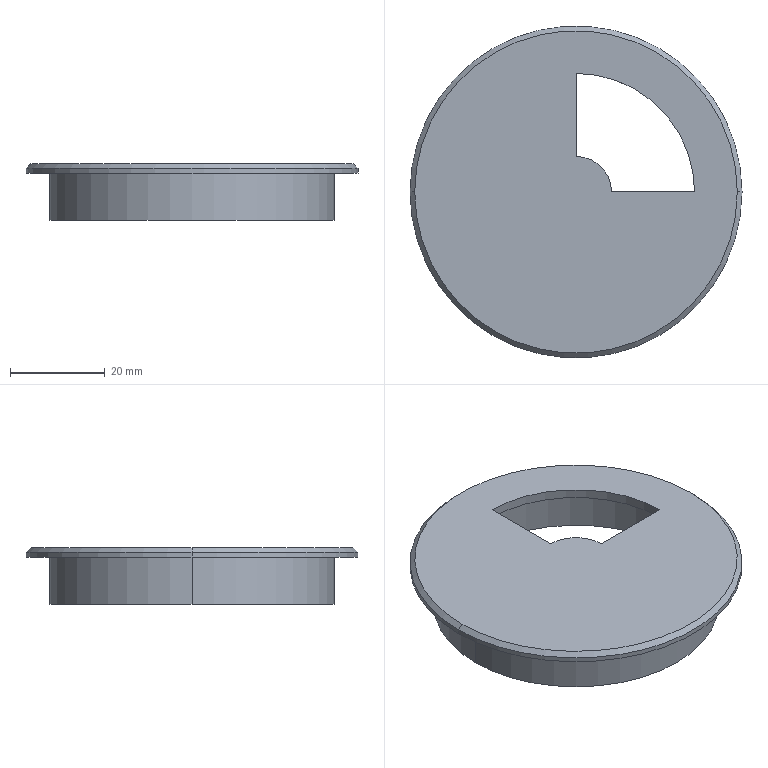Part | STEP file | 1 solid | 16 faces | box 70 x 70 x 12 mm | volume 8548 mm3 | cylinder 8 | plane 6 | cone 2 | commonest cylinder face diameters 58 x2 60 x2 70 x2 15 x1 50 x1
STEP:
#1=CARTESIAN_POINT('',(0.,0.,0.));
#2=DIRECTION('',(0.,0.,1.));
#3=DIRECTION('',(1.,0.,0.));
#4=AXIS2_PLACEMENT_3D('',#1,#2,#3);
#5=CARTESIAN_POINT('',(34.,0.,12.));
#6=VERTEX_POINT('',#5);
#7=CARTESIAN_POINT('',(-34.,0.,12.));
#8=VERTEX_POINT('',#7);
#9=CARTESIAN_POINT('',(0.,0.,12.));
#10=DIRECTION('',(0.,0.,1.));
#11=DIRECTION('',(1.,0.,0.));
#12=AXIS2_PLACEMENT_3D('',#9,#10,#11);
#13=CIRCLE('',#12,34.);
#14=CARTESIAN_POINT('',(0.,0.,12.));
#15=DIRECTION('',(0.,0.,-1.));
#16=DIRECTION('',(-1.,0.,0.));
#17=AXIS2_PLACEMENT_3D('',#14,#15,#16);
#18=CONICAL_SURFACE('',#17,34.,0.7854);
#19=CARTESIAN_POINT('',(3.142,0.));
#20=DIRECTION('',(-1.,0.));
#21=VECTOR('',#20,1.);
#22=LINE('',#19,#21);
#23=(GEOMETRIC_REPRESENTATION_CONTEXT(2)PARAMETRIC_REPRESENTATION_CONTEXT()REPRESENTATION_CONTEXT('',''));
#24=DEFINITIONAL_REPRESENTATION('',(#22),#23);
#25=PCURVE('',#18,#24);
#26=CARTESIAN_POINT('',(0.,0.,12.));
#27=DIRECTION('',(0.,0.,1.));
#28=DIRECTION('',(1.,0.,0.));
#29=AXIS2_PLACEMENT_3D('',#26,#27,#28);
#30=PLANE('',#29);
#31=CARTESIAN_POINT('',(0.,0.));
#32=DIRECTION('',(1.,0.));
#33=AXIS2_PLACEMENT_2D('',#31,#32);
#34=CIRCLE('',#33,34.);
#35=(GEOMETRIC_REPRESENTATION_CONTEXT(2)PARAMETRIC_REPRESENTATION_CONTEXT()REPRESENTATION_CONTEXT('',''));
#36=DEFINITIONAL_REPRESENTATION('',(#34),#35);
#37=PCURVE('',#30,#36);
#38=SURFACE_CURVE('',#13,(#25,#37),.PCURVE_S1.);
#39=EDGE_CURVE('',#6,#8,#38,.T.);
#40=ORIENTED_EDGE('',*,*,#39,.F.);
#41=CARTESIAN_POINT('',(35.,0.,11.));
#42=VERTEX_POINT('',#41);
#43=CARTESIAN_POINT('',(34.,0.,12.));
#44=DIRECTION('',(0.7071,0.,-0.7071));
#45=VECTOR('',#44,1.);
#46=LINE('',#43,#45);
#47=CARTESIAN_POINT('',(3.142,0.));
#48=DIRECTION('',(0.,1.));
#49=VECTOR('',#48,1.);
#50=LINE('',#47,#49);
#51=(GEOMETRIC_REPRESENTATION_CONTEXT(2)PARAMETRIC_REPRESENTATION_CONTEXT()REPRESENTATION_CONTEXT('',''));
#52=DEFINITIONAL_REPRESENTATION('',(#50),#51);
#53=PCURVE('',#18,#52);
#54=CARTESIAN_POINT('',(0.,0.,12.));
#55=DIRECTION('',(0.,0.,-1.));
#56=DIRECTION('',(-1.,0.,0.));
#57=AXIS2_PLACEMENT_3D('',#54,#55,#56);
#58=CONICAL_SURFACE('',#57,34.,0.7854);
#59=CARTESIAN_POINT('',(3.142,0.));
#60=DIRECTION('',(0.,1.));
#61=VECTOR('',#60,1.);
#62=LINE('',#59,#61);
#63=(GEOMETRIC_REPRESENTATION_CONTEXT(2)PARAMETRIC_REPRESENTATION_CONTEXT()REPRESENTATION_CONTEXT('',''));
#64=DEFINITIONAL_REPRESENTATION('',(#62),#63);
#65=PCURVE('',#58,#64);
#66=SURFACE_CURVE('',#46,(#53,#65),.PCURVE_S1.);
#67=EDGE_CURVE('',#6,#42,#66,.T.);
#68=ORIENTED_EDGE('',*,*,#67,.T.);
#69=CARTESIAN_POINT('',(-35.,0.,11.));
#70=VERTEX_POINT('',#69);
#71=CARTESIAN_POINT('',(0.,0.,11.));
#72=DIRECTION('',(0.,0.,-1.));
#73=DIRECTION('',(1.,0.,0.));
#74=AXIS2_PLACEMENT_3D('',#71,#72,#73);
#75=CIRCLE('',#74,35.);
#76=CARTESIAN_POINT('',(-3.142,1.));
#77=DIRECTION('',(1.,0.));
#78=VECTOR('',#77,1.);
#79=LINE('',#76,#78);
#80=(GEOMETRIC_REPRESENTATION_CONTEXT(2)PARAMETRIC_REPRESENTATION_CONTEXT()REPRESENTATION_CONTEXT('',''));
#81=DEFINITIONAL_REPRESENTATION('',(#79),#80);
#82=PCURVE('',#18,#81);
#83=CARTESIAN_POINT('',(0.,0.,12.));
#84=DIRECTION('',(0.,0.,-1.));
#85=DIRECTION('',(-1.,0.,0.));
#86=AXIS2_PLACEMENT_3D('',#83,#84,#85);
#87=CYLINDRICAL_SURFACE('',#86,35.);
#88=CARTESIAN_POINT('',(-3.142,1.));
#89=DIRECTION('',(1.,0.));
#90=VECTOR('',#89,1.);
#91=LINE('',#88,#90);
#92=(GEOMETRIC_REPRESENTATION_CONTEXT(2)PARAMETRIC_REPRESENTATION_CONTEXT()REPRESENTATION_CONTEXT('',''));
#93=DEFINITIONAL_REPRESENTATION('',(#91),#92);
#94=PCURVE('',#87,#93);
#95=SURFACE_CURVE('',#75,(#82,#94),.PCURVE_S1.);
#96=EDGE_CURVE('',#70,#42,#95,.T.);
#97=ORIENTED_EDGE('',*,*,#96,.F.);
#98=CARTESIAN_POINT('',(-34.,0.,12.));
#99=DIRECTION('',(-0.7071,0.,-0.7071));
#100=VECTOR('',#99,1.);
#101=LINE('',#98,#100);
#102=CARTESIAN_POINT('',(0.,0.));
#103=DIRECTION('',(0.,1.));
#104=VECTOR('',#103,1.);
#105=LINE('',#102,#104);
#106=(GEOMETRIC_REPRESENTATION_CONTEXT(2)PARAMETRIC_REPRESENTATION_CONTEXT()REPRESENTATION_CONTEXT('',''));
#107=DEFINITIONAL_REPRESENTATION('',(#105),#106);
#108=PCURVE('',#18,#107);
#109=CARTESIAN_POINT('',(6.283,0.));
#110=DIRECTION('',(0.,1.));
#111=VECTOR('',#110,1.);
#112=LINE('',#109,#111);
#113=(GEOMETRIC_REPRESENTATION_CONTEXT(2)PARAMETRIC_REPRESENTATION_CONTEXT()REPRESENTATION_CONTEXT('',''));
#114=DEFINITIONAL_REPRESENTATION('',(#112),#113);
#115=PCURVE('',#58,#114);
#116=SURFACE_CURVE('',#101,(#108,#115),.PCURVE_S1.);
#117=EDGE_CURVE('',#8,#70,#116,.T.);
#118=ORIENTED_EDGE('',*,*,#117,.F.);
#119=EDGE_LOOP('',(#40,#68,#97,#118));
#120=FACE_BOUND('',#119,.T.);
#121=ADVANCED_FACE('',(#120),#18,.T.);
#122=ORIENTED_EDGE('',*,*,#96,.T.);
#123=CARTESIAN_POINT('',(35.,0.,10.));
#124=VERTEX_POINT('',#123);
#125=CARTESIAN_POINT('',(35.,0.,12.));
#126=DIRECTION('',(0.,0.,-1.));
#127=VECTOR('',#126,1.);
#128=LINE('',#125,#127);
#129=CARTESIAN_POINT('',(3.142,0.));
#130=DIRECTION('',(0.,1.));
#131=VECTOR('',#130,1.);
#132=LINE('',#129,#131);
#133=(GEOMETRIC_REPRESENTATION_CONTEXT(2)PARAMETRIC_REPRESENTATION_CONTEXT()REPRESENTATION_CONTEXT('',''));
#134=DEFINITIONAL_REPRESENTATION('',(#132),#133);
#135=PCURVE('',#87,#134);
#136=CARTESIAN_POINT('',(0.,0.,12.));
#137=DIRECTION('',(0.,0.,-1.));
#138=DIRECTION('',(-1.,0.,0.));
#139=AXIS2_PLACEMENT_3D('',#136,#137,#138);
#140=CYLINDRICAL_SURFACE('',#139,35.);
#141=CARTESIAN_POINT('',(3.142,0.));
#142=DIRECTION('',(0.,1.));
#143=VECTOR('',#142,1.);
#144=LINE('',#141,#143);
#145=(GEOMETRIC_REPRESENTATION_CONTEXT(2)PARAMETRIC_REPRESENTATION_CONTEXT()REPRESENTATION_CONTEXT('',''));
#146=DEFINITIONAL_REPRESENTATION('',(#144),#145);
#147=PCURVE('',#140,#146);
#148=SURFACE_CURVE('',#128,(#135,#147),.PCURVE_S1.);
#149=EDGE_CURVE('',#42,#124,#148,.T.);
#150=ORIENTED_EDGE('',*,*,#149,.T.);
#151=CARTESIAN_POINT('',(-35.,0.,10.));
#152=VERTEX_POINT('',#151);
#153=CARTESIAN_POINT('',(0.,0.,10.));
#154=DIRECTION('',(0.,0.,1.));
#155=DIRECTION('',(1.,0.,0.));
#156=AXIS2_PLACEMENT_3D('',#153,#154,#155);
#157=CIRCLE('',#156,35.);
#158=CARTESIAN_POINT('',(3.142,2.));
#159=DIRECTION('',(-1.,0.));
#160=VECTOR('',#159,1.);
#161=LINE('',#158,#160);
#162=(GEOMETRIC_REPRESENTATION_CONTEXT(2)PARAMETRIC_REPRESENTATION_CONTEXT()REPRESENTATION_CONTEXT('',''));
#163=DEFINITIONAL_REPRESENTATION('',(#161),#162);
#164=PCURVE('',#87,#163);
#165=CARTESIAN_POINT('',(0.,0.,10.));
#166=DIRECTION('',(0.,0.,1.));
#167=DIRECTION('',(1.,0.,0.));
#168=AXIS2_PLACEMENT_3D('',#165,#166,#167);
#169=PLANE('',#168);
#170=CARTESIAN_POINT('',(0.,0.));
#171=DIRECTION('',(1.,0.));
#172=AXIS2_PLACEMENT_2D('',#170,#171);
#173=CIRCLE('',#172,35.);
#174=(GEOMETRIC_REPRESENTATION_CONTEXT(2)PARAMETRIC_REPRESENTATION_CONTEXT()REPRESENTATION_CONTEXT('',''));
#175=DEFINITIONAL_REPRESENTATION('',(#173),#174);
#176=PCURVE('',#169,#175);
#177=SURFACE_CURVE('',#157,(#164,#176),.PCURVE_S1.);
#178=EDGE_CURVE('',#124,#152,#177,.T.);
#179=ORIENTED_EDGE('',*,*,#178,.T.);
#180=CARTESIAN_POINT('',(-35.,0.,12.));
#181=DIRECTION('',(0.,0.,-1.));
#182=VECTOR('',#181,1.);
#183=LINE('',#180,#182);
#184=CARTESIAN_POINT('',(0.,0.));
#185=DIRECTION('',(0.,1.));
#186=VECTOR('',#185,1.);
#187=LINE('',#184,#186);
#188=(GEOMETRIC_REPRESENTATION_CONTEXT(2)PARAMETRIC_REPRESENTATION_CONTEXT()REPRESENTATION_CONTEXT('',''));
#189=DEFINITIONAL_REPRESENTATION('',(#187),#188);
#190=PCURVE('',#87,#189);
#191=CARTESIAN_POINT('',(6.283,0.));
#192=DIRECTION('',(0.,1.));
#193=VECTOR('',#192,1.);
#194=LINE('',#191,#193);
#195=(GEOMETRIC_REPRESENTATION_CONTEXT(2)PARAMETRIC_REPRESENTATION_CONTEXT()REPRESENTATION_CONTEXT('',''));
#196=DEFINITIONAL_REPRESENTATION('',(#194),#195);
#197=PCURVE('',#140,#196);
#198=SURFACE_CURVE('',#183,(#190,#197),.PCURVE_S1.);
#199=EDGE_CURVE('',#70,#152,#198,.T.);
#200=ORIENTED_EDGE('',*,*,#199,.F.);
#201=EDGE_LOOP('',(#122,#150,#179,#200));
#202=FACE_BOUND('',#201,.T.);
#203=ADVANCED_FACE('',(#202),#87,.T.);
#204=CARTESIAN_POINT('',(-29.,0.,10.));
#205=VERTEX_POINT('',#204);
#206=CARTESIAN_POINT('',(-29.,0.,0.));
#207=VERTEX_POINT('',#206);
#208=CARTESIAN_POINT('',(-29.,0.,10.));
#209=DIRECTION('',(0.,0.,-1.));
#210=VECTOR('',#209,1.);
#211=LINE('',#208,#210);
#212=CARTESIAN_POINT('',(0.,0.,10.));
#213=DIRECTION('',(0.,0.,-1.));
#214=DIRECTION('',(-1.,0.,0.));
#215=AXIS2_PLACEMENT_3D('',#212,#213,#214);
#216=CYLINDRICAL_SURFACE('',#215,29.);
#217=CARTESIAN_POINT('',(6.283,0.));
#218=DIRECTION('',(0.,1.));
#219=VECTOR('',#218,1.);
#220=LINE('',#217,#219);
#221=(GEOMETRIC_REPRESENTATION_CONTEXT(2)PARAMETRIC_REPRESENTATION_CONTEXT()REPRESENTATION_CONTEXT('',''));
#222=DEFINITIONAL_REPRESENTATION('',(#220),#221);
#223=PCURVE('',#216,#222);
#224=CARTESIAN_POINT('',(0.,0.,10.));
#225=DIRECTION('',(0.,0.,-1.));
#226=DIRECTION('',(-1.,0.,0.));
#227=AXIS2_PLACEMENT_3D('',#224,#225,#226);
#228=CYLINDRICAL_SURFACE('',#227,29.);
#229=CARTESIAN_POINT('',(0.,0.));
#230=DIRECTION('',(0.,1.));
#231=VECTOR('',#230,1.);
#232=LINE('',#229,#231);
#233=(GEOMETRIC_REPRESENTATION_CONTEXT(2)PARAMETRIC_REPRESENTATION_CONTEXT()REPRESENTATION_CONTEXT('',''));
#234=DEFINITIONAL_REPRESENTATION('',(#232),#233);
#235=PCURVE('',#228,#234);
#236=SURFACE_CURVE('',#211,(#223,#235),.PCURVE_S1.);
#237=EDGE_CURVE('',#205,#207,#236,.T.);
#238=ORIENTED_EDGE('',*,*,#237,.T.);
#239=CARTESIAN_POINT('',(29.,0.,0.));
#240=VERTEX_POINT('',#239);
#241=CARTESIAN_POINT('',(0.,0.,0.));
#242=DIRECTION('',(0.,0.,1.));
#243=DIRECTION('',(1.,0.,0.));
#244=AXIS2_PLACEMENT_3D('',#241,#242,#243);
#245=CIRCLE('',#244,29.);
#246=CARTESIAN_POINT('',(9.425,10.));
#247=DIRECTION('',(-1.,0.));
#248=VECTOR('',#247,1.);
#249=LINE('',#246,#248);
#250=(GEOMETRIC_REPRESENTATION_CONTEXT(2)PARAMETRIC_REPRESENTATION_CONTEXT()REPRESENTATION_CONTEXT('',''));
#251=DEFINITIONAL_REPRESENTATION('',(#249),#250);
#252=PCURVE('',#216,#251);
#253=CARTESIAN_POINT('',(0.,0.,0.));
#254=DIRECTION('',(0.,0.,1.));
#255=DIRECTION('',(1.,0.,0.));
#256=AXIS2_PLACEMENT_3D('',#253,#254,#255);
#257=PLANE('',#256);
#258=CARTESIAN_POINT('',(0.,0.));
#259=DIRECTION('',(1.,0.));
#260=AXIS2_PLACEMENT_2D('',#258,#259);
#261=CIRCLE('',#260,29.);
#262=(GEOMETRIC_REPRESENTATION_CONTEXT(2)PARAMETRIC_REPRESENTATION_CONTEXT()REPRESENTATION_CONTEXT('',''));
#263=DEFINITIONAL_REPRESENTATION('',(#261),#262);
#264=PCURVE('',#257,#263);
#265=SURFACE_CURVE('',#245,(#252,#264),.PCURVE_S1.);
#266=EDGE_CURVE('',#207,#240,#265,.T.);
#267=ORIENTED_EDGE('',*,*,#266,.T.);
#268=CARTESIAN_POINT('',(29.,0.,10.));
#269=VERTEX_POINT('',#268);
#270=CARTESIAN_POINT('',(29.,0.,10.));
#271=DIRECTION('',(0.,0.,-1.));
#272=VECTOR('',#271,1.);
#273=LINE('',#270,#272);
#274=CARTESIAN_POINT('',(3.142,0.));
#275=DIRECTION('',(0.,1.));
#276=VECTOR('',#275,1.);
#277=LINE('',#274,#276);
#278=(GEOMETRIC_REPRESENTATION_CONTEXT(2)PARAMETRIC_REPRESENTATION_CONTEXT()REPRESENTATION_CONTEXT('',''));
#279=DEFINITIONAL_REPRESENTATION('',(#277),#278);
#280=PCURVE('',#216,#279);
#281=CARTESIAN_POINT('',(3.142,0.));
#282=DIRECTION('',(0.,1.));
#283=VECTOR('',#282,1.);
#284=LINE('',#281,#283);
#285=(GEOMETRIC_REPRESENTATION_CONTEXT(2)PARAMETRIC_REPRESENTATION_CONTEXT()REPRESENTATION_CONTEXT('',''));
#286=DEFINITIONAL_REPRESENTATION('',(#284),#285);
#287=PCURVE('',#228,#286);
#288=SURFACE_CURVE('',#273,(#280,#287),.PCURVE_S1.);
#289=EDGE_CURVE('',#269,#240,#288,.T.);
#290=ORIENTED_EDGE('',*,*,#289,.F.);
#291=CARTESIAN_POINT('',(0.,0.,10.));
#292=DIRECTION('',(0.,0.,1.));
#293=DIRECTION('',(1.,0.,0.));
#294=AXIS2_PLACEMENT_3D('',#291,#292,#293);
#295=CIRCLE('',#294,29.);
#296=CARTESIAN_POINT('',(9.425,0.));
#297=DIRECTION('',(-1.,0.));
#298=VECTOR('',#297,1.);
#299=LINE('',#296,#298);
#300=(GEOMETRIC_REPRESENTATION_CONTEXT(2)PARAMETRIC_REPRESENTATION_CONTEXT()REPRESENTATION_CONTEXT('',''));
#301=DEFINITIONAL_REPRESENTATION('',(#299),#300);
#302=PCURVE('',#216,#301);
#303=CARTESIAN_POINT('',(0.,0.,10.));
#304=DIRECTION('',(0.,0.,1.));
#305=DIRECTION('',(1.,0.,0.));
#306=AXIS2_PLACEMENT_3D('',#303,#304,#305);
#307=PLANE('',#306);
#308=CARTESIAN_POINT('',(0.,0.));
#309=DIRECTION('',(1.,0.));
#310=AXIS2_PLACEMENT_2D('',#308,#309);
#311=CIRCLE('',#310,29.);
#312=(GEOMETRIC_REPRESENTATION_CONTEXT(2)PARAMETRIC_REPRESENTATION_CONTEXT()REPRESENTATION_CONTEXT('',''));
#313=DEFINITIONAL_REPRESENTATION('',(#311),#312);
#314=PCURVE('',#307,#313);
#315=SURFACE_CURVE('',#295,(#302,#314),.PCURVE_S1.);
#316=EDGE_CURVE('',#205,#269,#315,.T.);
#317=ORIENTED_EDGE('',*,*,#316,.F.);
#318=EDGE_LOOP('',(#238,#267,#290,#317));
#319=FACE_BOUND('',#318,.F.);
#320=ADVANCED_FACE('',(#319),#216,.F.);
#321=CARTESIAN_POINT('',(30.,0.,10.));
#322=VERTEX_POINT('',#321);
#323=CARTESIAN_POINT('',(-30.,0.,10.));
#324=VERTEX_POINT('',#323);
#325=CARTESIAN_POINT('',(0.,0.,10.));
#326=DIRECTION('',(0.,0.,1.));
#327=DIRECTION('',(1.,0.,0.));
#328=AXIS2_PLACEMENT_3D('',#325,#326,#327);
#329=CIRCLE('',#328,30.);
#330=CARTESIAN_POINT('',(0.,0.,10.));
#331=DIRECTION('',(0.,0.,-1.));
#332=DIRECTION('',(-1.,0.,0.));
#333=AXIS2_PLACEMENT_3D('',#330,#331,#332);
#334=CYLINDRICAL_SURFACE('',#333,30.);
#335=CARTESIAN_POINT('',(3.142,0.));
#336=DIRECTION('',(-1.,0.));
#337=VECTOR('',#336,1.);
#338=LINE('',#335,#337);
#339=(GEOMETRIC_REPRESENTATION_CONTEXT(2)PARAMETRIC_REPRESENTATION_CONTEXT()REPRESENTATION_CONTEXT('',''));
#340=DEFINITIONAL_REPRESENTATION('',(#338),#339);
#341=PCURVE('',#334,#340);
#342=CARTESIAN_POINT('',(0.,0.));
#343=DIRECTION('',(1.,0.));
#344=AXIS2_PLACEMENT_2D('',#342,#343);
#345=CIRCLE('',#344,30.);
#346=(GEOMETRIC_REPRESENTATION_CONTEXT(2)PARAMETRIC_REPRESENTATION_CONTEXT()REPRESENTATION_CONTEXT('',''));
#347=DEFINITIONAL_REPRESENTATION('',(#345),#346);
#348=PCURVE('',#169,#347);
#349=SURFACE_CURVE('',#329,(#341,#348),.PCURVE_S1.);
#350=EDGE_CURVE('',#322,#324,#349,.T.);
#351=ORIENTED_EDGE('',*,*,#350,.F.);
#352=CARTESIAN_POINT('',(30.,0.,0.));
#353=VERTEX_POINT('',#352);
#354=CARTESIAN_POINT('',(30.,0.,10.));
#355=DIRECTION('',(0.,0.,-1.));
#356=VECTOR('',#355,1.);
#357=LINE('',#354,#356);
#358=CARTESIAN_POINT('',(3.142,0.));
#359=DIRECTION('',(0.,1.));
#360=VECTOR('',#359,1.);
#361=LINE('',#358,#360);
#362=(GEOMETRIC_REPRESENTATION_CONTEXT(2)PARAMETRIC_REPRESENTATION_CONTEXT()REPRESENTATION_CONTEXT('',''));
#363=DEFINITIONAL_REPRESENTATION('',(#361),#362);
#364=PCURVE('',#334,#363);
#365=CARTESIAN_POINT('',(0.,0.,10.));
#366=DIRECTION('',(0.,0.,-1.));
#367=DIRECTION('',(-1.,0.,0.));
#368=AXIS2_PLACEMENT_3D('',#365,#366,#367);
#369=CYLINDRICAL_SURFACE('',#368,30.);
#370=CARTESIAN_POINT('',(3.142,0.));
#371=DIRECTION('',(0.,1.));
#372=VECTOR('',#371,1.);
#373=LINE('',#370,#372);
#374=(GEOMETRIC_REPRESENTATION_CONTEXT(2)PARAMETRIC_REPRESENTATION_CONTEXT()REPRESENTATION_CONTEXT('',''));
#375=DEFINITIONAL_REPRESENTATION('',(#373),#374);
#376=PCURVE('',#369,#375);
#377=SURFACE_CURVE('',#357,(#364,#376),.PCURVE_S1.);
#378=EDGE_CURVE('',#322,#353,#377,.T.);
#379=ORIENTED_EDGE('',*,*,#378,.T.);
#380=CARTESIAN_POINT('',(-30.,0.,0.));
#381=VERTEX_POINT('',#380);
#382=CARTESIAN_POINT('',(0.,0.,0.));
#383=DIRECTION('',(0.,0.,1.));
#384=DIRECTION('',(1.,0.,0.));
#385=AXIS2_PLACEMENT_3D('',#382,#383,#384);
#386=CIRCLE('',#385,30.);
#387=CARTESIAN_POINT('',(3.142,10.));
#388=DIRECTION('',(-1.,0.));
#389=VECTOR('',#388,1.);
#390=LINE('',#387,#389);
#391=(GEOMETRIC_REPRESENTATION_CONTEXT(2)PARAMETRIC_REPRESENTATION_CONTEXT()REPRESENTATION_CONTEXT('',''));
#392=DEFINITIONAL_REPRESENTATION('',(#390),#391);
#393=PCURVE('',#334,#392);
#394=CARTESIAN_POINT('',(0.,0.));
#395=DIRECTION('',(1.,0.));
#396=AXIS2_PLACEMENT_2D('',#394,#395);
#397=CIRCLE('',#396,30.);
#398=(GEOMETRIC_REPRESENTATION_CONTEXT(2)PARAMETRIC_REPRESENTATION_CONTEXT()REPRESENTATION_CONTEXT('',''));
#399=DEFINITIONAL_REPRESENTATION('',(#397),#398);
#400=PCURVE('',#257,#399);
#401=SURFACE_CURVE('',#386,(#393,#400),.PCURVE_S1.);
#402=EDGE_CURVE('',#353,#381,#401,.T.);
#403=ORIENTED_EDGE('',*,*,#402,.T.);
#404=CARTESIAN_POINT('',(-30.,0.,10.));
#405=DIRECTION('',(0.,0.,-1.));
#406=VECTOR('',#405,1.);
#407=LINE('',#404,#406);
#408=CARTESIAN_POINT('',(0.,0.));
#409=DIRECTION('',(0.,1.));
#410=VECTOR('',#409,1.);
#411=LINE('',#408,#410);
#412=(GEOMETRIC_REPRESENTATION_CONTEXT(2)PARAMETRIC_REPRESENTATION_CONTEXT()REPRESENTATION_CONTEXT('',''));
#413=DEFINITIONAL_REPRESENTATION('',(#411),#412);
#414=PCURVE('',#334,#413);
#415=CARTESIAN_POINT('',(6.283,0.));
#416=DIRECTION('',(0.,1.));
#417=VECTOR('',#416,1.);
#418=LINE('',#415,#417);
#419=(GEOMETRIC_REPRESENTATION_CONTEXT(2)PARAMETRIC_REPRESENTATION_CONTEXT()REPRESENTATION_CONTEXT('',''));
#420=DEFINITIONAL_REPRESENTATION('',(#418),#419);
#421=PCURVE('',#369,#420);
#422=SURFACE_CURVE('',#407,(#414,#421),.PCURVE_S1.);
#423=EDGE_CURVE('',#324,#381,#422,.T.);
#424=ORIENTED_EDGE('',*,*,#423,.F.);
#425=EDGE_LOOP('',(#351,#379,#403,#424));
#426=FACE_BOUND('',#425,.T.);
#427=ADVANCED_FACE('',(#426),#334,.T.);
#428=CARTESIAN_POINT('',(0.,0.,0.));
#429=DIRECTION('',(0.,0.,1.));
#430=DIRECTION('',(1.,0.,0.));
#431=AXIS2_PLACEMENT_3D('',#428,#429,#430);
#432=CIRCLE('',#431,30.);
#433=CARTESIAN_POINT('',(0.,0.));
#434=DIRECTION('',(1.,0.));
#435=AXIS2_PLACEMENT_2D('',#433,#434);
#436=CIRCLE('',#435,30.);
#437=(GEOMETRIC_REPRESENTATION_CONTEXT(2)PARAMETRIC_REPRESENTATION_CONTEXT()REPRESENTATION_CONTEXT('',''));
#438=DEFINITIONAL_REPRESENTATION('',(#436),#437);
#439=PCURVE('',#257,#438);
#440=CARTESIAN_POINT('',(9.425,10.));
#441=DIRECTION('',(-1.,0.));
#442=VECTOR('',#441,1.);
#443=LINE('',#440,#442);
#444=(GEOMETRIC_REPRESENTATION_CONTEXT(2)PARAMETRIC_REPRESENTATION_CONTEXT()REPRESENTATION_CONTEXT('',''));
#445=DEFINITIONAL_REPRESENTATION('',(#443),#444);
#446=PCURVE('',#369,#445);
#447=SURFACE_CURVE('',#432,(#439,#446),.PCURVE_S1.);
#448=EDGE_CURVE('',#381,#353,#447,.T.);
#449=ORIENTED_EDGE('',*,*,#448,.F.);
#450=ORIENTED_EDGE('',*,*,#402,.F.);
#451=EDGE_LOOP('',(#449,#450));
#452=FACE_BOUND('',#451,.T.);
#453=ORIENTED_EDGE('',*,*,#266,.T.);
#454=CARTESIAN_POINT('',(0.,0.,0.));
#455=DIRECTION('',(0.,0.,1.));
#456=DIRECTION('',(1.,0.,0.));
#457=AXIS2_PLACEMENT_3D('',#454,#455,#456);
#458=CIRCLE('',#457,29.);
#459=CARTESIAN_POINT('',(0.,0.));
#460=DIRECTION('',(1.,0.));
#461=AXIS2_PLACEMENT_2D('',#459,#460);
#462=CIRCLE('',#461,29.);
#463=(GEOMETRIC_REPRESENTATION_CONTEXT(2)PARAMETRIC_REPRESENTATION_CONTEXT()REPRESENTATION_CONTEXT('',''));
#464=DEFINITIONAL_REPRESENTATION('',(#462),#463);
#465=PCURVE('',#257,#464);
#466=CARTESIAN_POINT('',(3.142,10.));
#467=DIRECTION('',(-1.,0.));
#468=VECTOR('',#467,1.);
#469=LINE('',#466,#468);
#470=(GEOMETRIC_REPRESENTATION_CONTEXT(2)PARAMETRIC_REPRESENTATION_CONTEXT()REPRESENTATION_CONTEXT('',''));
#471=DEFINITIONAL_REPRESENTATION('',(#469),#470);
#472=PCURVE('',#228,#471);
#473=SURFACE_CURVE('',#458,(#465,#472),.PCURVE_S1.);
#474=EDGE_CURVE('',#240,#207,#473,.T.);
#475=ORIENTED_EDGE('',*,*,#474,.T.);
#476=EDGE_LOOP('',(#453,#475));
#477=FACE_BOUND('',#476,.T.);
#478=ADVANCED_FACE('',(#452,#477),#257,.F.);
#479=ORIENTED_EDGE('',*,*,#378,.F.);
#480=CARTESIAN_POINT('',(0.,0.,10.));
#481=DIRECTION('',(0.,0.,1.));
#482=DIRECTION('',(1.,0.,0.));
#483=AXIS2_PLACEMENT_3D('',#480,#481,#482);
#484=CIRCLE('',#483,30.);
#485=CARTESIAN_POINT('',(9.425,0.));
#486=DIRECTION('',(-1.,0.));
#487=VECTOR('',#486,1.);
#488=LINE('',#485,#487);
#489=(GEOMETRIC_REPRESENTATION_CONTEXT(2)PARAMETRIC_REPRESENTATION_CONTEXT()REPRESENTATION_CONTEXT('',''));
#490=DEFINITIONAL_REPRESENTATION('',(#488),#489);
#491=PCURVE('',#369,#490);
#492=CARTESIAN_POINT('',(0.,0.));
#493=DIRECTION('',(1.,0.));
#494=AXIS2_PLACEMENT_2D('',#492,#493);
#495=CIRCLE('',#494,30.);
#496=(GEOMETRIC_REPRESENTATION_CONTEXT(2)PARAMETRIC_REPRESENTATION_CONTEXT()REPRESENTATION_CONTEXT('',''));
#497=DEFINITIONAL_REPRESENTATION('',(#495),#496);
#498=PCURVE('',#169,#497);
#499=SURFACE_CURVE('',#484,(#491,#498),.PCURVE_S1.);
#500=EDGE_CURVE('',#324,#322,#499,.T.);
#501=ORIENTED_EDGE('',*,*,#500,.F.);
#502=ORIENTED_EDGE('',*,*,#423,.T.);
#503=ORIENTED_EDGE('',*,*,#448,.T.);
#504=EDGE_LOOP('',(#479,#501,#502,#503));
#505=FACE_BOUND('',#504,.T.);
#506=ADVANCED_FACE('',(#505),#369,.T.);
#507=ORIENTED_EDGE('',*,*,#474,.T.);
#508=ORIENTED_EDGE('',*,*,#237,.F.);
#509=CARTESIAN_POINT('',(0.,0.,10.));
#510=DIRECTION('',(0.,0.,1.));
#511=DIRECTION('',(1.,0.,0.));
#512=AXIS2_PLACEMENT_3D('',#509,#510,#511);
#513=CIRCLE('',#512,29.);
#514=CARTESIAN_POINT('',(3.142,0.));
#515=DIRECTION('',(-1.,0.));
#516=VECTOR('',#515,1.);
#517=LINE('',#514,#516);
#518=(GEOMETRIC_REPRESENTATION_CONTEXT(2)PARAMETRIC_REPRESENTATION_CONTEXT()REPRESENTATION_CONTEXT('',''));
#519=DEFINITIONAL_REPRESENTATION('',(#517),#518);
#520=PCURVE('',#228,#519);
#521=CARTESIAN_POINT('',(0.,0.));
#522=DIRECTION('',(1.,0.));
#523=AXIS2_PLACEMENT_2D('',#521,#522);
#524=CIRCLE('',#523,29.);
#525=(GEOMETRIC_REPRESENTATION_CONTEXT(2)PARAMETRIC_REPRESENTATION_CONTEXT()REPRESENTATION_CONTEXT('',''));
#526=DEFINITIONAL_REPRESENTATION('',(#524),#525);
#527=PCURVE('',#307,#526);
#528=SURFACE_CURVE('',#513,(#520,#527),.PCURVE_S1.);
#529=EDGE_CURVE('',#269,#205,#528,.T.);
#530=ORIENTED_EDGE('',*,*,#529,.F.);
#531=ORIENTED_EDGE('',*,*,#289,.T.);
#532=EDGE_LOOP('',(#507,#508,#530,#531));
#533=FACE_BOUND('',#532,.F.);
#534=ADVANCED_FACE('',(#533),#228,.F.);
#535=CARTESIAN_POINT('',(0.,25.,10.));
#536=VERTEX_POINT('',#535);
#537=CARTESIAN_POINT('',(0.,7.5,10.));
#538=VERTEX_POINT('',#537);
#539=CARTESIAN_POINT('',(0.,25.,10.));
#540=DIRECTION('',(0.,-1.,0.));
#541=VECTOR('',#540,1.);
#542=LINE('',#539,#541);
#543=CARTESIAN_POINT('',(0.,25.));
#544=DIRECTION('',(0.,-1.));
#545=VECTOR('',#544,1.);
#546=LINE('',#543,#545);
#547=(GEOMETRIC_REPRESENTATION_CONTEXT(2)PARAMETRIC_REPRESENTATION_CONTEXT()REPRESENTATION_CONTEXT('',''));
#548=DEFINITIONAL_REPRESENTATION('',(#546),#547);
#549=PCURVE('',#307,#548);
#550=CARTESIAN_POINT('',(0.,25.,10.));
#551=DIRECTION('',(-1.,0.,0.));
#552=DIRECTION('',(0.,-1.,0.));
#553=AXIS2_PLACEMENT_3D('',#550,#551,#552);
#554=PLANE('',#553);
#555=CARTESIAN_POINT('',(0.,0.));
#556=DIRECTION('',(1.,0.));
#557=VECTOR('',#556,1.);
#558=LINE('',#555,#557);
#559=(GEOMETRIC_REPRESENTATION_CONTEXT(2)PARAMETRIC_REPRESENTATION_CONTEXT()REPRESENTATION_CONTEXT('',''));
#560=DEFINITIONAL_REPRESENTATION('',(#558),#559);
#561=PCURVE('',#554,#560);
#562=SURFACE_CURVE('',#542,(#549,#561),.PCURVE_S1.);
#563=EDGE_CURVE('',#536,#538,#562,.T.);
#564=ORIENTED_EDGE('',*,*,#563,.T.);
#565=CARTESIAN_POINT('',(7.5,0.,10.));
#566=VERTEX_POINT('',#565);
#567=CARTESIAN_POINT('',(0.,0.,10.));
#568=DIRECTION('',(0.,0.,1.));
#569=DIRECTION('',(1.,0.,0.));
#570=AXIS2_PLACEMENT_3D('',#567,#568,#569);
#571=CIRCLE('',#570,7.5);
#572=CARTESIAN_POINT('',(0.,0.));
#573=DIRECTION('',(1.,0.));
#574=AXIS2_PLACEMENT_2D('',#572,#573);
#575=CIRCLE('',#574,7.5);
#576=(GEOMETRIC_REPRESENTATION_CONTEXT(2)PARAMETRIC_REPRESENTATION_CONTEXT()REPRESENTATION_CONTEXT('',''));
#577=DEFINITIONAL_REPRESENTATION('',(#575),#576);
#578=PCURVE('',#307,#577);
#579=CARTESIAN_POINT('',(0.,0.,10.));
#580=DIRECTION('',(0.,0.,1.));
#581=DIRECTION('',(1.,0.,0.));
#582=AXIS2_PLACEMENT_3D('',#579,#580,#581);
#583=CYLINDRICAL_SURFACE('',#582,7.5);
#584=CARTESIAN_POINT('',(0.,0.));
#585=DIRECTION('',(1.,0.));
#586=VECTOR('',#585,1.);
#587=LINE('',#584,#586);
#588=(GEOMETRIC_REPRESENTATION_CONTEXT(2)PARAMETRIC_REPRESENTATION_CONTEXT()REPRESENTATION_CONTEXT('',''));
#589=DEFINITIONAL_REPRESENTATION('',(#587),#588);
#590=PCURVE('',#583,#589);
#591=SURFACE_CURVE('',#571,(#578,#590),.PCURVE_S1.);
#592=EDGE_CURVE('',#566,#538,#591,.T.);
#593=ORIENTED_EDGE('',*,*,#592,.F.);
#594=CARTESIAN_POINT('',(25.,0.,10.));
#595=VERTEX_POINT('',#594);
#596=CARTESIAN_POINT('',(0.,0.,10.));
#597=DIRECTION('',(1.,0.,0.));
#598=VECTOR('',#597,1.);
#599=LINE('',#596,#598);
#600=CARTESIAN_POINT('',(0.,0.));
#601=DIRECTION('',(1.,0.));
#602=VECTOR('',#601,1.);
#603=LINE('',#600,#602);
#604=(GEOMETRIC_REPRESENTATION_CONTEXT(2)PARAMETRIC_REPRESENTATION_CONTEXT()REPRESENTATION_CONTEXT('',''));
#605=DEFINITIONAL_REPRESENTATION('',(#603),#604);
#606=PCURVE('',#307,#605);
#607=CARTESIAN_POINT('',(0.,0.,10.));
#608=DIRECTION('',(0.,-1.,0.));
#609=DIRECTION('',(0.,0.,-1.));
#610=AXIS2_PLACEMENT_3D('',#607,#608,#609);
#611=PLANE('',#610);
#612=CARTESIAN_POINT('',(0.,0.));
#613=DIRECTION('',(0.,1.));
#614=VECTOR('',#613,1.);
#615=LINE('',#612,#614);
#616=(GEOMETRIC_REPRESENTATION_CONTEXT(2)PARAMETRIC_REPRESENTATION_CONTEXT()REPRESENTATION_CONTEXT('',''));
#617=DEFINITIONAL_REPRESENTATION('',(#615),#616);
#618=PCURVE('',#611,#617);
#619=SURFACE_CURVE('',#599,(#606,#618),.PCURVE_S1.);
#620=EDGE_CURVE('',#566,#595,#619,.T.);
#621=ORIENTED_EDGE('',*,*,#620,.T.);
#622=CARTESIAN_POINT('',(0.,0.,10.));
#623=DIRECTION('',(0.,0.,1.));
#624=DIRECTION('',(-1.,0.,0.));
#625=AXIS2_PLACEMENT_3D('',#622,#623,#624);
#626=CIRCLE('',#625,25.);
#627=CARTESIAN_POINT('',(0.,0.));
#628=DIRECTION('',(-1.,0.));
#629=AXIS2_PLACEMENT_2D('',#627,#628);
#630=CIRCLE('',#629,25.);
#631=(GEOMETRIC_REPRESENTATION_CONTEXT(2)PARAMETRIC_REPRESENTATION_CONTEXT()REPRESENTATION_CONTEXT('',''));
#632=DEFINITIONAL_REPRESENTATION('',(#630),#631);
#633=PCURVE('',#307,#632);
#634=CARTESIAN_POINT('',(0.,0.,10.));
#635=DIRECTION('',(0.,0.,1.));
#636=DIRECTION('',(1.,0.,0.));
#637=AXIS2_PLACEMENT_3D('',#634,#635,#636);
#638=CYLINDRICAL_SURFACE('',#637,25.);
#639=CARTESIAN_POINT('',(-3.142,0.));
#640=DIRECTION('',(1.,0.));
#641=VECTOR('',#640,1.);
#642=LINE('',#639,#641);
#643=(GEOMETRIC_REPRESENTATION_CONTEXT(2)PARAMETRIC_REPRESENTATION_CONTEXT()REPRESENTATION_CONTEXT('',''));
#644=DEFINITIONAL_REPRESENTATION('',(#642),#643);
#645=PCURVE('',#638,#644);
#646=SURFACE_CURVE('',#626,(#633,#645),.PCURVE_S1.);
#647=EDGE_CURVE('',#595,#536,#646,.T.);
#648=ORIENTED_EDGE('',*,*,#647,.T.);
#649=EDGE_LOOP('',(#564,#593,#621,#648));
#650=FACE_BOUND('',#649,.T.);
#651=ORIENTED_EDGE('',*,*,#316,.F.);
#652=ORIENTED_EDGE('',*,*,#529,.F.);
#653=EDGE_LOOP('',(#651,#652));
#654=FACE_BOUND('',#653,.T.);
#655=ADVANCED_FACE('',(#650,#654),#307,.F.);
#656=CARTESIAN_POINT('',(0.,0.,10.));
#657=DIRECTION('',(0.,0.,1.));
#658=DIRECTION('',(1.,0.,0.));
#659=AXIS2_PLACEMENT_3D('',#656,#657,#658);
#660=CIRCLE('',#659,35.);
#661=CARTESIAN_POINT('',(0.,0.));
#662=DIRECTION('',(1.,0.));
#663=AXIS2_PLACEMENT_2D('',#661,#662);
#664=CIRCLE('',#663,35.);
#665=(GEOMETRIC_REPRESENTATION_CONTEXT(2)PARAMETRIC_REPRESENTATION_CONTEXT()REPRESENTATION_CONTEXT('',''));
#666=DEFINITIONAL_REPRESENTATION('',(#664),#665);
#667=PCURVE('',#169,#666);
#668=CARTESIAN_POINT('',(9.425,2.));
#669=DIRECTION('',(-1.,0.));
#670=VECTOR('',#669,1.);
#671=LINE('',#668,#670);
#672=(GEOMETRIC_REPRESENTATION_CONTEXT(2)PARAMETRIC_REPRESENTATION_CONTEXT()REPRESENTATION_CONTEXT('',''));
#673=DEFINITIONAL_REPRESENTATION('',(#671),#672);
#674=PCURVE('',#140,#673);
#675=SURFACE_CURVE('',#660,(#667,#674),.PCURVE_S1.);
#676=EDGE_CURVE('',#152,#124,#675,.T.);
#677=ORIENTED_EDGE('',*,*,#676,.F.);
#678=ORIENTED_EDGE('',*,*,#178,.F.);
#679=EDGE_LOOP('',(#677,#678));
#680=FACE_BOUND('',#679,.T.);
#681=ORIENTED_EDGE('',*,*,#500,.T.);
#682=ORIENTED_EDGE('',*,*,#350,.T.);
#683=EDGE_LOOP('',(#681,#682));
#684=FACE_BOUND('',#683,.T.);
#685=ADVANCED_FACE('',(#680,#684),#169,.F.);
#686=ORIENTED_EDGE('',*,*,#149,.F.);
#687=CARTESIAN_POINT('',(0.,0.,11.));
#688=DIRECTION('',(0.,0.,-1.));
#689=DIRECTION('',(1.,0.,0.));
#690=AXIS2_PLACEMENT_3D('',#687,#688,#689);
#691=CIRCLE('',#690,35.);
#692=CARTESIAN_POINT('',(3.142,1.));
#693=DIRECTION('',(1.,0.));
#694=VECTOR('',#693,1.);
#695=LINE('',#692,#694);
#696=(GEOMETRIC_REPRESENTATION_CONTEXT(2)PARAMETRIC_REPRESENTATION_CONTEXT()REPRESENTATION_CONTEXT('',''));
#697=DEFINITIONAL_REPRESENTATION('',(#695),#696);
#698=PCURVE('',#140,#697);
#699=CARTESIAN_POINT('',(3.142,1.));
#700=DIRECTION('',(1.,0.));
#701=VECTOR('',#700,1.);
#702=LINE('',#699,#701);
#703=(GEOMETRIC_REPRESENTATION_CONTEXT(2)PARAMETRIC_REPRESENTATION_CONTEXT()REPRESENTATION_CONTEXT('',''));
#704=DEFINITIONAL_REPRESENTATION('',(#702),#703);
#705=PCURVE('',#58,#704);
#706=SURFACE_CURVE('',#691,(#698,#705),.PCURVE_S1.);
#707=EDGE_CURVE('',#42,#70,#706,.T.);
#708=ORIENTED_EDGE('',*,*,#707,.T.);
#709=ORIENTED_EDGE('',*,*,#199,.T.);
#710=ORIENTED_EDGE('',*,*,#676,.T.);
#711=EDGE_LOOP('',(#686,#708,#709,#710));
#712=FACE_BOUND('',#711,.T.);
#713=ADVANCED_FACE('',(#712),#140,.T.);
#714=CARTESIAN_POINT('',(0.,0.,12.));
#715=DIRECTION('',(0.,0.,1.));
#716=DIRECTION('',(1.,0.,0.));
#717=AXIS2_PLACEMENT_3D('',#714,#715,#716);
#718=CIRCLE('',#717,34.);
#719=CARTESIAN_POINT('',(0.,0.));
#720=DIRECTION('',(1.,0.));
#721=AXIS2_PLACEMENT_2D('',#719,#720);
#722=CIRCLE('',#721,34.);
#723=(GEOMETRIC_REPRESENTATION_CONTEXT(2)PARAMETRIC_REPRESENTATION_CONTEXT()REPRESENTATION_CONTEXT('',''));
#724=DEFINITIONAL_REPRESENTATION('',(#722),#723);
#725=PCURVE('',#30,#724);
#726=CARTESIAN_POINT('',(9.425,0.));
#727=DIRECTION('',(-1.,0.));
#728=VECTOR('',#727,1.);
#729=LINE('',#726,#728);
#730=(GEOMETRIC_REPRESENTATION_CONTEXT(2)PARAMETRIC_REPRESENTATION_CONTEXT()REPRESENTATION_CONTEXT('',''));
#731=DEFINITIONAL_REPRESENTATION('',(#729),#730);
#732=PCURVE('',#58,#731);
#733=SURFACE_CURVE('',#718,(#725,#732),.PCURVE_S1.);
#734=EDGE_CURVE('',#8,#6,#733,.T.);
#735=ORIENTED_EDGE('',*,*,#734,.T.);
#736=ORIENTED_EDGE('',*,*,#39,.T.);
#737=EDGE_LOOP('',(#735,#736));
#738=FACE_BOUND('',#737,.T.);
#739=CARTESIAN_POINT('',(7.5,0.,12.));
#740=VERTEX_POINT('',#739);
#741=CARTESIAN_POINT('',(25.,0.,12.));
#742=VERTEX_POINT('',#741);
#743=CARTESIAN_POINT('',(0.,0.,12.));
#744=DIRECTION('',(1.,0.,0.));
#745=VECTOR('',#744,1.);
#746=LINE('',#743,#745);
#747=CARTESIAN_POINT('',(0.,0.));
#748=DIRECTION('',(1.,0.));
#749=VECTOR('',#748,1.);
#750=LINE('',#747,#749);
#751=(GEOMETRIC_REPRESENTATION_CONTEXT(2)PARAMETRIC_REPRESENTATION_CONTEXT()REPRESENTATION_CONTEXT('',''));
#752=DEFINITIONAL_REPRESENTATION('',(#750),#751);
#753=PCURVE('',#30,#752);
#754=CARTESIAN_POINT('',(-2.,0.));
#755=DIRECTION('',(0.,1.));
#756=VECTOR('',#755,1.);
#757=LINE('',#754,#756);
#758=(GEOMETRIC_REPRESENTATION_CONTEXT(2)PARAMETRIC_REPRESENTATION_CONTEXT()REPRESENTATION_CONTEXT('',''));
#759=DEFINITIONAL_REPRESENTATION('',(#757),#758);
#760=PCURVE('',#611,#759);
#761=SURFACE_CURVE('',#746,(#753,#760),.PCURVE_S1.);
#762=EDGE_CURVE('',#740,#742,#761,.T.);
#763=ORIENTED_EDGE('',*,*,#762,.F.);
#764=CARTESIAN_POINT('',(0.,7.5,12.));
#765=VERTEX_POINT('',#764);
#766=CARTESIAN_POINT('',(0.,0.,12.));
#767=DIRECTION('',(0.,0.,1.));
#768=DIRECTION('',(1.,0.,0.));
#769=AXIS2_PLACEMENT_3D('',#766,#767,#768);
#770=CIRCLE('',#769,7.5);
#771=CARTESIAN_POINT('',(0.,0.));
#772=DIRECTION('',(1.,0.));
#773=AXIS2_PLACEMENT_2D('',#771,#772);
#774=CIRCLE('',#773,7.5);
#775=(GEOMETRIC_REPRESENTATION_CONTEXT(2)PARAMETRIC_REPRESENTATION_CONTEXT()REPRESENTATION_CONTEXT('',''));
#776=DEFINITIONAL_REPRESENTATION('',(#774),#775);
#777=PCURVE('',#30,#776);
#778=CARTESIAN_POINT('',(0.,2.));
#779=DIRECTION('',(1.,0.));
#780=VECTOR('',#779,1.);
#781=LINE('',#778,#780);
#782=(GEOMETRIC_REPRESENTATION_CONTEXT(2)PARAMETRIC_REPRESENTATION_CONTEXT()REPRESENTATION_CONTEXT('',''));
#783=DEFINITIONAL_REPRESENTATION('',(#781),#782);
#784=PCURVE('',#583,#783);
#785=SURFACE_CURVE('',#770,(#777,#784),.PCURVE_S1.);
#786=EDGE_CURVE('',#740,#765,#785,.T.);
#787=ORIENTED_EDGE('',*,*,#786,.T.);
#788=CARTESIAN_POINT('',(0.,25.,12.));
#789=VERTEX_POINT('',#788);
#790=CARTESIAN_POINT('',(0.,25.,12.));
#791=DIRECTION('',(0.,-1.,0.));
#792=VECTOR('',#791,1.);
#793=LINE('',#790,#792);
#794=CARTESIAN_POINT('',(0.,25.));
#795=DIRECTION('',(0.,-1.));
#796=VECTOR('',#795,1.);
#797=LINE('',#794,#796);
#798=(GEOMETRIC_REPRESENTATION_CONTEXT(2)PARAMETRIC_REPRESENTATION_CONTEXT()REPRESENTATION_CONTEXT('',''));
#799=DEFINITIONAL_REPRESENTATION('',(#797),#798);
#800=PCURVE('',#30,#799);
#801=CARTESIAN_POINT('',(0.,2.));
#802=DIRECTION('',(1.,0.));
#803=VECTOR('',#802,1.);
#804=LINE('',#801,#803);
#805=(GEOMETRIC_REPRESENTATION_CONTEXT(2)PARAMETRIC_REPRESENTATION_CONTEXT()REPRESENTATION_CONTEXT('',''));
#806=DEFINITIONAL_REPRESENTATION('',(#804),#805);
#807=PCURVE('',#554,#806);
#808=SURFACE_CURVE('',#793,(#800,#807),.PCURVE_S1.);
#809=EDGE_CURVE('',#789,#765,#808,.T.);
#810=ORIENTED_EDGE('',*,*,#809,.F.);
#811=CARTESIAN_POINT('',(0.,0.,12.));
#812=DIRECTION('',(0.,0.,1.));
#813=DIRECTION('',(-1.,0.,0.));
#814=AXIS2_PLACEMENT_3D('',#811,#812,#813);
#815=CIRCLE('',#814,25.);
#816=CARTESIAN_POINT('',(0.,0.));
#817=DIRECTION('',(-1.,0.));
#818=AXIS2_PLACEMENT_2D('',#816,#817);
#819=CIRCLE('',#818,25.);
#820=(GEOMETRIC_REPRESENTATION_CONTEXT(2)PARAMETRIC_REPRESENTATION_CONTEXT()REPRESENTATION_CONTEXT('',''));
#821=DEFINITIONAL_REPRESENTATION('',(#819),#820);
#822=PCURVE('',#30,#821);
#823=CARTESIAN_POINT('',(-3.142,2.));
#824=DIRECTION('',(1.,0.));
#825=VECTOR('',#824,1.);
#826=LINE('',#823,#825);
#827=(GEOMETRIC_REPRESENTATION_CONTEXT(2)PARAMETRIC_REPRESENTATION_CONTEXT()REPRESENTATION_CONTEXT('',''));
#828=DEFINITIONAL_REPRESENTATION('',(#826),#827);
#829=PCURVE('',#638,#828);
#830=SURFACE_CURVE('',#815,(#822,#829),.PCURVE_S1.);
#831=EDGE_CURVE('',#742,#789,#830,.T.);
#832=ORIENTED_EDGE('',*,*,#831,.F.);
#833=EDGE_LOOP('',(#763,#787,#810,#832));
#834=FACE_BOUND('',#833,.T.);
#835=ADVANCED_FACE('',(#738,#834),#30,.T.);
#836=ORIENTED_EDGE('',*,*,#620,.F.);
#837=CARTESIAN_POINT('',(7.5,0.,10.));
#838=DIRECTION('',(0.,0.,1.));
#839=VECTOR('',#838,1.);
#840=LINE('',#837,#839);
#841=CARTESIAN_POINT('',(0.,7.5));
#842=DIRECTION('',(-1.,0.));
#843=VECTOR('',#842,1.);
#844=LINE('',#841,#843);
#845=(GEOMETRIC_REPRESENTATION_CONTEXT(2)PARAMETRIC_REPRESENTATION_CONTEXT()REPRESENTATION_CONTEXT('',''));
#846=DEFINITIONAL_REPRESENTATION('',(#844),#845);
#847=PCURVE('',#611,#846);
#848=CARTESIAN_POINT('',(0.,0.));
#849=DIRECTION('',(0.,1.));
#850=VECTOR('',#849,1.);
#851=LINE('',#848,#850);
#852=(GEOMETRIC_REPRESENTATION_CONTEXT(2)PARAMETRIC_REPRESENTATION_CONTEXT()REPRESENTATION_CONTEXT('',''));
#853=DEFINITIONAL_REPRESENTATION('',(#851),#852);
#854=PCURVE('',#583,#853);
#855=SURFACE_CURVE('',#840,(#847,#854),.PCURVE_S1.);
#856=EDGE_CURVE('',#566,#740,#855,.T.);
#857=ORIENTED_EDGE('',*,*,#856,.T.);
#858=ORIENTED_EDGE('',*,*,#762,.T.);
#859=CARTESIAN_POINT('',(25.,0.,10.));
#860=DIRECTION('',(0.,0.,1.));
#861=VECTOR('',#860,1.);
#862=LINE('',#859,#861);
#863=CARTESIAN_POINT('',(0.,25.));
#864=DIRECTION('',(-1.,0.));
#865=VECTOR('',#864,1.);
#866=LINE('',#863,#865);
#867=(GEOMETRIC_REPRESENTATION_CONTEXT(2)PARAMETRIC_REPRESENTATION_CONTEXT()REPRESENTATION_CONTEXT('',''));
#868=DEFINITIONAL_REPRESENTATION('',(#866),#867);
#869=PCURVE('',#611,#868);
#870=CARTESIAN_POINT('',(0.,0.));
#871=DIRECTION('',(0.,1.));
#872=VECTOR('',#871,1.);
#873=LINE('',#870,#872);
#874=(GEOMETRIC_REPRESENTATION_CONTEXT(2)PARAMETRIC_REPRESENTATION_CONTEXT()REPRESENTATION_CONTEXT('',''));
#875=DEFINITIONAL_REPRESENTATION('',(#873),#874);
#876=PCURVE('',#638,#875);
#877=SURFACE_CURVE('',#862,(#869,#876),.PCURVE_S1.);
#878=EDGE_CURVE('',#595,#742,#877,.T.);
#879=ORIENTED_EDGE('',*,*,#878,.F.);
#880=EDGE_LOOP('',(#836,#857,#858,#879));
#881=FACE_BOUND('',#880,.T.);
#882=ADVANCED_FACE('',(#881),#611,.F.);
#883=ORIENTED_EDGE('',*,*,#809,.T.);
#884=CARTESIAN_POINT('',(0.,7.5,10.));
#885=DIRECTION('',(0.,0.,-1.));
#886=VECTOR('',#885,1.);
#887=LINE('',#884,#886);
#888=CARTESIAN_POINT('',(17.5,0.));
#889=DIRECTION('',(0.,-1.));
#890=VECTOR('',#889,1.);
#891=LINE('',#888,#890);
#892=(GEOMETRIC_REPRESENTATION_CONTEXT(2)PARAMETRIC_REPRESENTATION_CONTEXT()REPRESENTATION_CONTEXT('',''));
#893=DEFINITIONAL_REPRESENTATION('',(#891),#892);
#894=PCURVE('',#554,#893);
#895=CARTESIAN_POINT('',(1.571,0.));
#896=DIRECTION('',(0.,-1.));
#897=VECTOR('',#896,1.);
#898=LINE('',#895,#897);
#899=(GEOMETRIC_REPRESENTATION_CONTEXT(2)PARAMETRIC_REPRESENTATION_CONTEXT()REPRESENTATION_CONTEXT('',''));
#900=DEFINITIONAL_REPRESENTATION('',(#898),#899);
#901=PCURVE('',#583,#900);
#902=SURFACE_CURVE('',#887,(#894,#901),.PCURVE_S1.);
#903=EDGE_CURVE('',#765,#538,#902,.T.);
#904=ORIENTED_EDGE('',*,*,#903,.T.);
#905=ORIENTED_EDGE('',*,*,#563,.F.);
#906=CARTESIAN_POINT('',(0.,25.,10.));
#907=DIRECTION('',(0.,0.,1.));
#908=VECTOR('',#907,1.);
#909=LINE('',#906,#908);
#910=CARTESIAN_POINT('',(0.,0.));
#911=DIRECTION('',(0.,1.));
#912=VECTOR('',#911,1.);
#913=LINE('',#910,#912);
#914=(GEOMETRIC_REPRESENTATION_CONTEXT(2)PARAMETRIC_REPRESENTATION_CONTEXT()REPRESENTATION_CONTEXT('',''));
#915=DEFINITIONAL_REPRESENTATION('',(#913),#914);
#916=PCURVE('',#554,#915);
#917=CARTESIAN_POINT('',(1.571,0.));
#918=DIRECTION('',(0.,1.));
#919=VECTOR('',#918,1.);
#920=LINE('',#917,#919);
#921=(GEOMETRIC_REPRESENTATION_CONTEXT(2)PARAMETRIC_REPRESENTATION_CONTEXT()REPRESENTATION_CONTEXT('',''));
#922=DEFINITIONAL_REPRESENTATION('',(#920),#921);
#923=PCURVE('',#638,#922);
#924=SURFACE_CURVE('',#909,(#916,#923),.PCURVE_S1.);
#925=EDGE_CURVE('',#536,#789,#924,.T.);
#926=ORIENTED_EDGE('',*,*,#925,.T.);
#927=EDGE_LOOP('',(#883,#904,#905,#926));
#928=FACE_BOUND('',#927,.T.);
#929=ADVANCED_FACE('',(#928),#554,.F.);
#930=ORIENTED_EDGE('',*,*,#878,.F.);
#931=ORIENTED_EDGE('',*,*,#647,.T.);
#932=ORIENTED_EDGE('',*,*,#925,.T.);
#933=ORIENTED_EDGE('',*,*,#831,.F.);
#934=EDGE_LOOP('',(#930,#931,#932,#933));
#935=FACE_BOUND('',#934,.F.);
#936=ADVANCED_FACE('',(#935),#638,.F.);
#937=ORIENTED_EDGE('',*,*,#856,.F.);
#938=ORIENTED_EDGE('',*,*,#592,.T.);
#939=ORIENTED_EDGE('',*,*,#903,.F.);
#940=ORIENTED_EDGE('',*,*,#786,.F.);
#941=EDGE_LOOP('',(#937,#938,#939,#940));
#942=FACE_BOUND('',#941,.T.);
#943=ADVANCED_FACE('',(#942),#583,.T.);
#944=ORIENTED_EDGE('',*,*,#67,.F.);
#945=ORIENTED_EDGE('',*,*,#734,.F.);
#946=ORIENTED_EDGE('',*,*,#117,.T.);
#947=ORIENTED_EDGE('',*,*,#707,.F.);
#948=EDGE_LOOP('',(#944,#945,#946,#947));
#949=FACE_BOUND('',#948,.T.);
#950=ADVANCED_FACE('',(#949),#58,.T.);
#951=CLOSED_SHELL('',(#121,#203,#320,#427,#478,#506,#534,#655,#685,#713,#835,#882,#929,#936,#943,#950));
#952=MANIFOLD_SOLID_BREP('',#951);
#953=(LENGTH_UNIT()NAMED_UNIT(*)SI_UNIT(.MILLI.,.METRE.));
#954=UNCERTAINTY_MEASURE_WITH_UNIT(LENGTH_MEASURE(0.0000001),#953,'','');
#955=(NAMED_UNIT(*)PLANE_ANGLE_UNIT()SI_UNIT($,.RADIAN.));
#956=(NAMED_UNIT(*)SI_UNIT($,.STERADIAN.)SOLID_ANGLE_UNIT());
#957=(GEOMETRIC_REPRESENTATION_CONTEXT(3)GLOBAL_UNCERTAINTY_ASSIGNED_CONTEXT((#954))GLOBAL_UNIT_ASSIGNED_CONTEXT((#953,#955,#956))REPRESENTATION_CONTEXT('',''));
#958=ADVANCED_BREP_SHAPE_REPRESENTATION('',(#4,#952),#957);